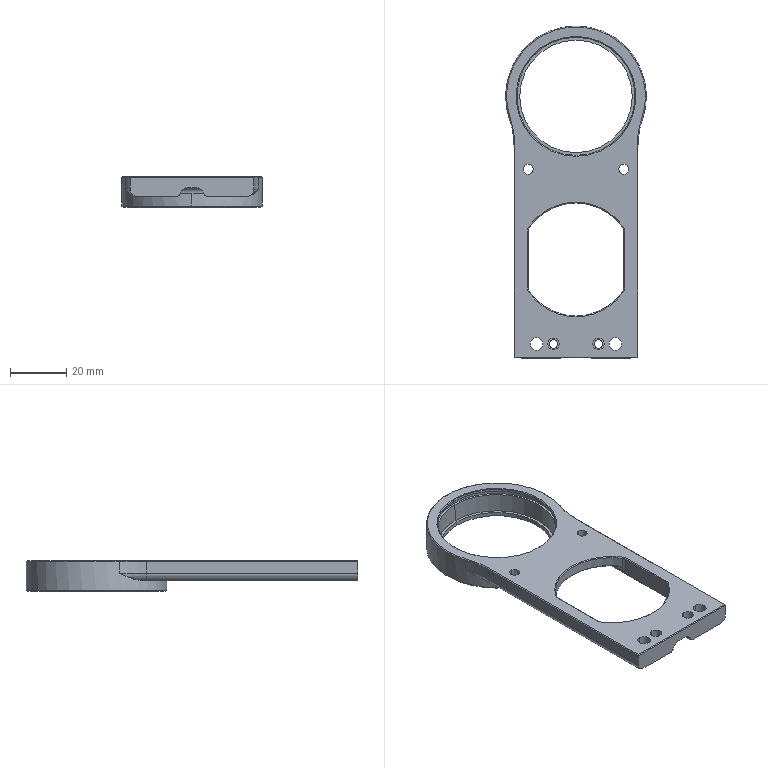NC program | NX | posted with a generic post | part box 50 x 118 x 11 mm
Lines 2350 to 3723 of 3723:
(ZLEVEL_PROFILE_COPY , TOOL : D10JING)
N4680 T14 M6
N4682 G54
N4684 G17 G0 G90 X-64. Y1.257 S9500 M3
N4686 G43 Z30. H14
N4688 Z-9.5
N4690 G94 G1 Y22.549 Z-10.616 F1000.
N4692 X-63.672 Y23.864 Z-10.687
N4694 X-63.004 Y25.045 Z-10.758
N4696 X-62.045 Y26.004 Z-10.829
N4698 X-60.864 Y26.672 Z-10.9
N4700 X-59.549 Y27. Z-10.971
N4702 X-59. Z-11.
N4704 X16.084 F1500.
N4706 G3 X24.227 Y28.364 R25.
N4708 G2 X24.227 Y-28.364 R-30.
N4710 G3 X16.084 Y-27. R25.
N4712 G1 X-59.
N4714 G2 X-64. Y-22. R5.
N4716 G1 Y22.
N4718 G2 X-59. Y27. R5.
N4720 G1 Z-9.5
N4722 G0 Z30.
(ZLEVEL_PROFILE_COPY_1_COPY , TOOL : D10JING)
N4724 X-15.695 Y-12.
N4726 Z-9.
N4728 G1 X-14.834 Z-9.045 F1000.
N4730 X-14.077 Y-11.422 Z-9.095
N4732 X-12.278 Y-9.566 Z-9.231
N4734 X-10.82 Y-7.43 Z-9.366
N4736 X-9.747 Y-5.077 Z-9.502
N4738 X-9.091 Y-2.576 Z-9.637
N4740 X-8.87 Y0. Z-9.773
N4742 X-9.091 Y2.576 Z-9.908
N4744 X-9.747 Y5.077 Z-10.044
N4746 X-10.82 Y7.43 Z-10.179
N4748 X-12.278 Y9.566 Z-10.315
N4750 X-14.077 Y11.422 Z-10.45
N4752 X-14.834 Y12. Z-10.5
N4754 X-33.166 F1500.
N4756 G3 X-33.166 Y-12. R15.1
N4758 G1 X-14.834
N4760 G3 X-14.834 Y12. R15.1
N4762 G1 Z-9.
N4764 G0 Z30.
(HOLE_MILLING_COPY_COPY , TOOL : D10JING)
N4766 X34. Y0.
N4768 Z0.5
N4770 G41 G1 X33.901 Y0.016 F1000. D14
N4772 G3 X34. Y-16.005 R8.011
N4774 X34. Y-16.005 Z-0.5 I0. J16.005 F2000.
N4776 X34. Y-16.005 Z-1.5 I0. J16.005
N4778 X34. Y-16.005 Z-2.5 I0. J16.005
N4780 X34. Y-16.005 Z-3.5 I0. J16.005
N4782 X34. Y-16.005 Z-4.5 I0. J16.005
N4784 X34. Y-16.005 Z-5.5 I0. J16.005
N4786 X34. Y-16.005 Z-6.5 I0. J16.005
N4788 X34. Y-16.005 Z-7.5 I0. J16.005
N4790 X34. Y-16.005 Z-8.5 I0. J16.005
N4792 X34. Y-16.005 Z-9.5 I0. J16.005
N4794 X36.504 Y-15.808 Z-9.525 R16.005
N4796 X49.808 Y2.504 R16.005
N4798 X36.504 Y-15.808 R-16.005
N4800 X34.095 Y0.031 R8.011
N4802 G40
N4804 G1 X34. Y0.
N4806 G0 Z30.
(HOLE_MILLING_COPY_COPY_COPY , TOOL : D10JING)
N4808 Z0.25
N4810 G1 X30.606 Y-11.51 F1000.
N4812 G3 X34. Y-16.05 R3.539
N4814 X34. Y-16.05 Z-0.75 I0. J16.05 F2000.
N4816 X50.05 Y0. Z-1. R16.05
N4818 X34. Y16.05 R16.05
N4820 X50.05 Y0. R-16.05
N4822 X45.51 Y3.394 R3.539
N4824 G1 X34. Y0.
N4826 G0 Z30.
N4828 M5
(SPOT_DRILLING , TOOL : D6A45)
N4830 T01 M6
N4832 G54
N4834 G17 G0 G90 X8.084 Y17. S9500 M3
N4836 G43 Z30. H1
N4838 G94 G82 G98 Z-1. F250. P200 R3.
N4840 X34. Y0.
N4842 X8.084 Y-17.
N4844 X-54. Y-14.
N4846 Y-8.
N4848 Y8.
N4850 Y14.
N4852 G80
N4854 G0 X-54. Y14. Z30.
N4856 M5
(DRILLING , TOOL : 4.5ZT)
N4858 T08 M6
N4860 G54
N4862 G17 G0 G90 X-54. Y14. S2500 M3
N4864 G43 Z30. H8
N4866 G94 G83 G98 Z-6.452 F200. Q2. R3.
N4868 Y-14.
N4870 G80
N4872 G0 X-54. Y-14. Z30.
N4874 M5
(DRILLING_COPY , TOOL : 3.0ZT)
N4876 T16 M6
N4878 G54
N4880 G17 G0 G90 X-54. Y8. S2500 M3
N4882 G43 Z30. H16
N4884 G94 G83 G98 Z-9.401 F200. Q2. R3.
N4886 Y-8.
N4888 G80
N4890 G0 X-54. Y-8. Z30.
N4892 M5
(DRILLING_COPY_COPY , TOOL : 3.5ZT)
N4894 T07 M6
N4896 G54
N4898 G17 G0 G90 X8.084 Y17. S2500 M3
N4900 G43 Z30. H7
N4902 G94 G83 G98 Z-9.521 F200. Q2. R3.
N4904 Y-17.
N4906 G80
N4908 G0 X8.084 Y-17. Z30.
N4910 M5
(ZLEVEL_PROFILE_COPY_1_COPY_1 , TOOL : D4)
N4912 T11 M6
N4914 G54
N4916 G17 G0 G90 X-34.931 Y-13.409 S9500 M3
N4918 G43 Z30. H11
N4920 Z0.808
N4922 G94 G1 Z-0.692 F1000.
N4924 X-35.016 Y-14.113
N4926 G3 X-34.859 Y-14.481 R0.4
N4928 X-34.13 Y-15. R18.1 F2000.
N4930 G1 X-33.269
N4932 G3 X-32.922 Y-14.8 R0.4
N4934 G1 X-32.576 Y-14.2
N4936 Z0.808
N4938 G0 X-34.931 Y-13.409 Z0.415
N4940 G1 Z-1.085 F1000.
N4942 X-35.016 Y-14.113
N4944 G3 X-34.859 Y-14.481 R0.4
N4946 X-34.13 Y-15. R18.1 F2000.
N4948 G1 X-33.269
N4950 G3 X-32.922 Y-14.8 R0.4
N4952 G1 X-32.576 Y-14.2
N4954 Z0.415
N4956 G0 X-34.931 Y-13.409 Z0.023
N4958 G1 Z-1.477 F1000.
N4960 X-35.016 Y-14.113
N4962 G3 X-34.859 Y-14.481 R0.4
N4964 X-34.13 Y-15. R18.1 F2000.
N4966 G1 X-33.269
N4968 G3 X-32.922 Y-14.8 R0.4
N4970 G1 X-32.576 Y-14.2
N4972 Z0.023
N4974 G0 X-34.931 Y-13.409 Z-0.369
N4976 G1 Z-1.869 F1000.
N4978 X-35.016 Y-14.113
N4980 G3 X-34.859 Y-14.481 R0.4
N4982 X-34.13 Y-15. R18.1 F2000.
N4984 G1 X-33.269
N4986 G3 X-32.922 Y-14.8 R0.4
N4988 G1 X-32.576 Y-14.2
N4990 Z-0.369
N4992 G0 X-34.931 Y-13.409 Z-0.762
N4994 G1 Z-2.262 F1000.
N4996 X-35.016 Y-14.113
N4998 G3 X-34.859 Y-14.481 R0.4
N5000 X-34.13 Y-15. R18.1 F2000.
N5002 G1 X-33.269
N5004 G3 X-32.922 Y-14.8 R0.4
N5006 G1 X-32.576 Y-14.2
N5008 Z-0.762
N5010 G0 X-34.931 Y-13.409 Z-1.154
N5012 G1 Z-2.654 F1000.
N5014 X-35.016 Y-14.113
N5016 G3 X-34.859 Y-14.481 R0.4
N5018 X-34.13 Y-15. R18.1 F2000.
N5020 G1 X-33.269
N5022 G3 X-32.922 Y-14.8 R0.4
N5024 G1 X-32.576 Y-14.2
N5026 Z-1.154
N5028 G0 X-34.931 Y-13.409 Z-1.546
N5030 G1 Z-3.046 F1000.
N5032 X-35.016 Y-14.113
N5034 G3 X-34.859 Y-14.481 R0.4
N5036 X-34.13 Y-15. R18.1 F2000.
N5038 G1 X-33.269
N5040 G3 X-32.922 Y-14.8 R0.4
N5042 G1 X-32.576 Y-14.2
N5044 Z-1.546
N5046 G0 X-34.931 Y-13.409 Z-1.938
N5048 G1 Z-3.438 F1000.
N5050 X-35.016 Y-14.113
N5052 G3 X-34.859 Y-14.481 R0.4
N5054 X-34.13 Y-15. R18.1 F2000.
N5056 G1 X-33.269
N5058 G3 X-32.922 Y-14.8 R0.4
N5060 G1 X-32.576 Y-14.2
N5062 Z-1.938
N5064 G0 X-34.931 Y-13.409 Z-2.331
N5066 G1 Z-3.831 F1000.
N5068 X-35.016 Y-14.113
N5070 G3 X-34.859 Y-14.481 R0.4
N5072 X-34.13 Y-15. R18.1 F2000.
N5074 G1 X-33.269
N5076 G3 X-32.922 Y-14.8 R0.4
N5078 G1 X-32.576 Y-14.2
N5080 Z-2.331
N5082 G0 X-34.931 Y-13.409 Z-2.723
N5084 G1 Z-4.223 F1000.
N5086 X-35.016 Y-14.113
N5088 G3 X-34.859 Y-14.481 R0.4
N5090 X-34.13 Y-15. R18.1 F2000.
N5092 G1 X-33.269
N5094 G3 X-32.922 Y-14.8 R0.4
N5096 G1 X-32.576 Y-14.2
N5098 Z-2.723
N5100 G0 X-34.931 Y-13.409 Z-3.115
N5102 G1 Z-4.615 F1000.
N5104 X-35.016 Y-14.113
N5106 G3 X-34.859 Y-14.481 R0.4
N5108 X-34.13 Y-15. R18.1 F2000.
N5110 G1 X-33.269
N5112 G3 X-32.922 Y-14.8 R0.4
N5114 G1 X-32.576 Y-14.2
N5116 Z-3.115
N5118 G0 X-34.931 Y-13.409 Z-3.508
N5120 G1 Z-5.008 F1000.
N5122 X-35.016 Y-14.113
N5124 G3 X-34.859 Y-14.481 R0.4
N5126 X-34.13 Y-15. R18.1 F2000.
N5128 G1 X-33.269
N5130 G3 X-32.922 Y-14.8 R0.4
N5132 G1 X-32.576 Y-14.2
N5134 Z-3.508
N5136 G0 X-34.931 Y-13.409 Z-3.9
N5138 G1 Z-5.4 F1000.
N5140 X-35.016 Y-14.113
N5142 G3 X-34.859 Y-14.481 R0.4
N5144 X-34.13 Y-15. R18.1 F2000.
N5146 G1 X-33.269
N5148 G3 X-32.922 Y-14.8 R0.4
N5150 G1 X-32.576 Y-14.2
N5152 Z-3.9
N5154 G0 X-34.931 Y-13.409 Z-4.292
N5156 G1 Z-5.792 F1000.
N5158 X-35.016 Y-14.113
N5160 G3 X-34.859 Y-14.481 R0.4
N5162 X-34.13 Y-15. R18.1 F2000.
N5164 G1 X-33.269
N5166 G3 X-32.922 Y-14.8 R0.4
N5168 G1 X-32.576 Y-14.2
N5170 Z-4.292
N5172 G0 X-34.931 Y-13.409 Z-4.685
N5174 G1 Z-6.185 F1000.
N5176 X-35.016 Y-14.113
N5178 G3 X-34.859 Y-14.481 R0.4
N5180 X-34.13 Y-15. R18.1 F2000.
N5182 G1 X-33.269
N5184 G3 X-32.922 Y-14.8 R0.4
N5186 G1 X-32.576 Y-14.2
N5188 Z-4.685
N5190 G0 X-34.931 Y-13.409 Z-5.077
N5192 G1 Z-6.577 F1000.
N5194 X-35.016 Y-14.113
N5196 G3 X-34.859 Y-14.481 R0.4
N5198 X-34.13 Y-15. R18.1 F2000.
N5200 G1 X-33.269
N5202 G3 X-32.922 Y-14.8 R0.4
N5204 G1 X-32.576 Y-14.2
N5206 Z-5.077
N5208 G0 X-34.939 Y-13.403 Z-5.469
N5210 G1 Z-6.969 F1000.
N5212 X-35.024 Y-14.107
N5214 G3 X-34.867 Y-14.475 R0.4
N5216 X-34.135 Y-14.997 R18.1 F2000.
N5218 G1 X-34.089 Y-15.
N5220 X-33.265
N5222 G3 X-32.918 Y-14.8 R0.4
N5224 G1 X-32.572 Y-14.2
N5226 Z-5.469
N5228 G0 X-34.939 Y-13.403 Z-5.862
N5230 G1 Z-7.362 F1000.
N5232 X-35.024 Y-14.107
N5234 G3 X-34.867 Y-14.475 R0.4
N5236 X-34.135 Y-14.997 R18.1 F2000.
N5238 G1 X-34.089 Y-15.
N5240 X-33.265
N5242 G3 X-32.918 Y-14.8 R0.4
N5244 G1 X-32.572 Y-14.2
N5246 Z-5.862
N5248 G0 X-34.939 Y-13.403 Z-6.254
N5250 G1 Z-7.754 F1000.
N5252 X-35.024 Y-14.107
N5254 G3 X-34.867 Y-14.475 R0.4
N5256 X-34.135 Y-14.997 R18.1 F2000.
N5258 G1 X-34.089 Y-15.
N5260 X-33.265
N5262 G3 X-32.918 Y-14.8 R0.4
N5264 G1 X-32.572 Y-14.2
N5266 Z-6.254
N5268 G0 X-34.939 Y-13.403 Z-6.646
N5270 G1 Z-8.146 F1000.
N5272 X-35.024 Y-14.107
N5274 G3 X-34.867 Y-14.475 R0.4
N5276 X-34.135 Y-14.997 R18.1 F2000.
N5278 G1 X-34.089 Y-15.
N5280 X-33.265
N5282 G3 X-32.918 Y-14.8 R0.4
N5284 G1 X-32.572 Y-14.2
N5286 Z-6.646
N5288 G0 X-34.939 Y-13.403 Z-7.038
N5290 G1 Z-8.538 F1000.
N5292 X-35.024 Y-14.107
N5294 G3 X-34.867 Y-14.475 R0.4
N5296 X-34.135 Y-14.997 R18.1 F2000.
N5298 G1 X-34.089 Y-15.
N5300 X-33.265
N5302 G3 X-32.918 Y-14.8 R0.4
N5304 G1 X-32.572 Y-14.2
N5306 Z-7.038
N5308 G0 X-34.939 Y-13.403 Z-7.431
N5310 G1 Z-8.931 F1000.
N5312 X-35.024 Y-14.107
N5314 G3 X-34.867 Y-14.475 R0.4
N5316 X-34.135 Y-14.997 R18.1 F2000.
N5318 G1 X-34.089 Y-15.
N5320 X-33.265
N5322 G3 X-32.918 Y-14.8 R0.4
N5324 G1 X-32.572 Y-14.2
N5326 Z-7.431
N5328 G0 X-34.939 Y-13.403 Z-7.823
N5330 G1 Z-9.323 F1000.
N5332 X-35.024 Y-14.107
N5334 G3 X-34.867 Y-14.475 R0.4
N5336 X-34.135 Y-14.997 R18.1 F2000.
N5338 G1 X-34.089 Y-15.
N5340 X-33.265
N5342 G3 X-32.918 Y-14.8 R0.4
N5344 G1 X-32.572 Y-14.2
N5346 Z-7.823
N5348 G0 X-34.939 Y-13.403 Z-8.215
N5350 G1 Z-9.715 F1000.
N5352 X-35.024 Y-14.107
N5354 G3 X-34.867 Y-14.475 R0.4
N5356 X-34.135 Y-14.997 R18.1 F2000.
N5358 G1 X-34.089 Y-15.
N5360 X-33.265
N5362 G3 X-32.918 Y-14.8 R0.4
N5364 G1 X-32.572 Y-14.2
N5366 Z-8.215
N5368 G0 X-34.939 Y-13.403 Z-8.608
N5370 G1 Z-10.108 F1000.
N5372 X-35.024 Y-14.107
N5374 G3 X-34.867 Y-14.475 R0.4
N5376 X-34.135 Y-14.997 R18.1 F2000.
N5378 G1 X-34.089 Y-15.
N5380 X-33.265
N5382 G3 X-32.918 Y-14.8 R0.4
N5384 G1 X-32.572 Y-14.2
N5386 Z-8.608
N5388 G0 X-34.939 Y-13.403 Z-9.
N5390 G1 Z-10.5 F1000.
N5392 X-35.024 Y-14.107
N5394 G3 X-34.867 Y-14.475 R0.4
N5396 X-34.135 Y-14.997 R18.1 F2000.
N5398 G1 X-34.089 Y-15.
N5400 X-33.265
N5402 G3 X-32.918 Y-14.8 R0.4
N5404 G1 X-32.572 Y-14.2
N5406 Z-9.
N5408 G0 Z30.
N5410 X-15.424
N5412 Z0.808
N5414 G1 Z-0.692 F1000.
N5416 X-15.078 Y-14.8
N5418 G3 X-14.731 Y-15. R0.4
N5420 G1 X-13.87 F2000.
N5422 G3 X-13.141 Y-14.481 R18.1
N5424 X-12.984 Y-14.113 R0.4
N5426 G1 X-13.069 Y-13.409
N5428 Z0.808
N5430 G0 X-15.424 Y-14.2 Z0.415
N5432 G1 Z-1.085 F1000.
N5434 X-15.078 Y-14.8
N5436 G3 X-14.731 Y-15. R0.4
N5438 G1 X-13.87 F2000.
N5440 G3 X-13.141 Y-14.481 R18.1
N5442 X-12.984 Y-14.113 R0.4
N5444 G1 X-13.069 Y-13.409
N5446 Z0.415
N5448 G0 X-15.424 Y-14.2 Z0.023
N5450 G1 Z-1.477 F1000.
N5452 X-15.078 Y-14.8
N5454 G3 X-14.731 Y-15. R0.4
N5456 G1 X-13.87 F2000.
N5458 G3 X-13.141 Y-14.481 R18.1
N5460 X-12.984 Y-14.113 R0.4
N5462 G1 X-13.069 Y-13.409
N5464 Z0.023
N5466 G0 X-15.424 Y-14.2 Z-0.369
N5468 G1 Z-1.869 F1000.
N5470 X-15.078 Y-14.8
N5472 G3 X-14.731 Y-15. R0.4
N5474 G1 X-13.87 F2000.
N5476 G3 X-13.141 Y-14.481 R18.1
N5478 X-12.984 Y-14.113 R0.4
N5480 G1 X-13.069 Y-13.409
N5482 Z-0.369
N5484 G0 X-15.424 Y-14.2 Z-0.762
N5486 G1 Z-2.262 F1000.
N5488 X-15.078 Y-14.8
N5490 G3 X-14.731 Y-15. R0.4
N5492 G1 X-13.87 F2000.
N5494 G3 X-13.141 Y-14.481 R18.1
N5496 X-12.984 Y-14.113 R0.4
N5498 G1 X-13.069 Y-13.409
N5500 Z-0.762
N5502 G0 X-15.424 Y-14.2 Z-1.154
N5504 G1 Z-2.654 F1000.
N5506 X-15.078 Y-14.8
N5508 G3 X-14.731 Y-15. R0.4
N5510 G1 X-13.87 F2000.
N5512 G3 X-13.141 Y-14.481 R18.1
N5514 X-12.984 Y-14.113 R0.4
N5516 G1 X-13.069 Y-13.409
N5518 Z-1.154
N5520 G0 X-15.424 Y-14.2 Z-1.546
N5522 G1 Z-3.046 F1000.
N5524 X-15.078 Y-14.8
N5526 G3 X-14.731 Y-15. R0.4
N5528 G1 X-13.87 F2000.
N5530 G3 X-13.141 Y-14.481 R18.1
N5532 X-12.984 Y-14.113 R0.4
N5534 G1 X-13.069 Y-13.409
N5536 Z-1.546
N5538 G0 X-15.424 Y-14.2 Z-1.938
N5540 G1 Z-3.438 F1000.
N5542 X-15.078 Y-14.8
N5544 G3 X-14.731 Y-15. R0.4
N5546 G1 X-13.87 F2000.
N5548 G3 X-13.141 Y-14.481 R18.1
N5550 X-12.984 Y-14.113 R0.4
N5552 G1 X-13.069 Y-13.409
N5554 Z-1.938
N5556 G0 X-15.424 Y-14.2 Z-2.331
N5558 G1 Z-3.831 F1000.
N5560 X-15.078 Y-14.8
N5562 G3 X-14.731 Y-15. R0.4
N5564 G1 X-13.87 F2000.
N5566 G3 X-13.141 Y-14.481 R18.1
N5568 X-12.984 Y-14.113 R0.4
N5570 G1 X-13.069 Y-13.409
N5572 Z-2.331
N5574 G0 X-15.424 Y-14.2 Z-2.723
N5576 G1 Z-4.223 F1000.
N5578 X-15.078 Y-14.8
N5580 G3 X-14.731 Y-15. R0.4
N5582 G1 X-13.87 F2000.
N5584 G3 X-13.141 Y-14.481 R18.1
N5586 X-12.984 Y-14.113 R0.4
N5588 G1 X-13.069 Y-13.409
N5590 Z-2.723
N5592 G0 X-15.424 Y-14.2 Z-3.115
N5594 G1 Z-4.615 F1000.
N5596 X-15.078 Y-14.8
N5598 G3 X-14.731 Y-15. R0.4
N5600 G1 X-13.87 F2000.
N5602 G3 X-13.141 Y-14.481 R18.1
N5604 X-12.984 Y-14.113 R0.4
N5606 G1 X-13.069 Y-13.409
N5608 Z-3.115
N5610 G0 X-15.424 Y-14.2 Z-3.508
N5612 G1 Z-5.008 F1000.
N5614 X-15.078 Y-14.8
N5616 G3 X-14.731 Y-15. R0.4
N5618 G1 X-13.87 F2000.
N5620 X-13.863 Y-14.995
N5622 G3 X-13.141 Y-14.481 R18.1
N5624 X-12.984 Y-14.113 R0.4
N5626 G1 X-13.069 Y-13.409
N5628 Z-3.508
N5630 G0 X-15.424 Y-14.2 Z-3.9
N5632 G1 Z-5.4 F1000.
N5634 X-15.078 Y-14.8
N5636 G3 X-14.731 Y-15. R0.4
N5638 G1 X-13.871 F2000.
N5640 X-13.867 Y-14.998
N5642 G3 X-13.141 Y-14.481 R18.1
N5644 X-12.984 Y-14.113 R0.4
N5646 G1 X-13.069 Y-13.409
N5648 Z-3.9
N5650 G0 X-15.424 Y-14.2 Z-4.292
N5652 G1 Z-5.792 F1000.
N5654 X-15.078 Y-14.8
N5656 G3 X-14.731 Y-15. R0.4
N5658 G1 X-13.868 Y-14.998 F2000.
N5660 G3 X-13.141 Y-14.481 R18.1
N5662 X-12.984 Y-14.113 R0.4
N5664 G1 X-13.069 Y-13.409
N5666 Z-4.292
N5668 G0 X-15.424 Y-14.2 Z-4.685
N5670 G1 Z-6.185 F1000.
N5672 X-15.078 Y-14.8
N5674 G3 X-14.731 Y-15. R0.4
N5676 G1 X-13.871 F2000.
N5678 X-13.868 Y-14.998
N5680 G3 X-13.141 Y-14.481 R18.1
N5682 X-12.984 Y-14.113 R0.4
N5684 G1 X-13.069 Y-13.409
N5686 Z-4.685
N5688 G0 X-15.424 Y-14.2 Z-5.077
N5690 G1 Z-6.577 F1000.
N5692 X-15.078 Y-14.8
N5694 G3 X-14.731 Y-15. R0.4
N5696 G1 X-13.906 F2000.
N5698 X-13.868 Y-14.999
N5700 G3 X-13.141 Y-14.481 R18.1
N5702 X-12.984 Y-14.113 R0.4
N5704 G1 X-13.069 Y-13.409
N5706 Z-5.077
N5708 G0 X-15.421 Y-14.2 Z-5.469
N5710 G1 Z-6.969 F1000.
N5712 X-15.075 Y-14.8
N5714 G3 X-14.728 Y-15. R0.4
N5716 G1 X-13.868 Y-14.999 F2000.
N5718 G3 X-13.146 Y-14.485 R18.1
N5720 X-12.989 Y-14.117 R0.4
N5722 G1 X-13.074 Y-13.413
N5724 Z-5.469
N5726 G0 X-15.421 Y-14.2 Z-5.862
N5728 G1 Z-7.362 F1000.
N5730 X-15.075 Y-14.8
N5732 G3 X-14.728 Y-15. R0.4
N5734 G1 X-13.868 Y-14.999 F2000.
N5736 G3 X-13.146 Y-14.485 R18.1
N5738 X-12.989 Y-14.117 R0.4
N5740 G1 X-13.074 Y-13.413
N5742 Z-5.862
N5744 G0 X-15.421 Y-14.2 Z-6.254
N5746 G1 Z-7.754 F1000.
N5748 X-15.075 Y-14.8
N5750 G3 X-14.728 Y-15. R0.4
N5752 G1 X-13.868 Y-14.999 F2000.
N5754 G3 X-13.146 Y-14.485 R18.1
N5756 X-12.989 Y-14.117 R0.4
N5758 G1 X-13.074 Y-13.413
N5760 Z-6.254
N5762 G0 X-15.421 Y-14.2 Z-6.646
N5764 G1 Z-8.146 F1000.
N5766 X-15.075 Y-14.8
N5768 G3 X-14.728 Y-15. R0.4
N5770 G1 X-13.868 Y-14.999 F2000.
N5772 G3 X-13.146 Y-14.485 R18.1
N5774 X-12.989 Y-14.117 R0.4
N5776 G1 X-13.074 Y-13.413
N5778 Z-6.646
N5780 G0 X-15.421 Y-14.2 Z-7.038
N5782 G1 Z-8.538 F1000.
N5784 X-15.075 Y-14.8
N5786 G3 X-14.728 Y-15. R0.4
N5788 G1 X-13.868 Y-14.999 F2000.
N5790 G3 X-13.146 Y-14.485 R18.1
N5792 X-12.989 Y-14.117 R0.4
N5794 G1 X-13.074 Y-13.413
N5796 Z-7.038
N5798 G0 X-15.421 Y-14.2 Z-7.431
N5800 G1 Z-8.931 F1000.
N5802 X-15.075 Y-14.8
N5804 G3 X-14.728 Y-15. R0.4
N5806 G1 X-13.868 Y-14.999 F2000.
N5808 G3 X-13.146 Y-14.485 R18.1
N5810 X-12.989 Y-14.117 R0.4
N5812 G1 X-13.074 Y-13.413
N5814 Z-7.431
N5816 G0 X-15.421 Y-14.2 Z-7.823
N5818 G1 Z-9.323 F1000.
N5820 X-15.075 Y-14.8
N5822 G3 X-14.728 Y-15. R0.4
N5824 G1 X-13.868 Y-14.999 F2000.
N5826 G3 X-13.146 Y-14.485 R18.1
N5828 X-12.989 Y-14.117 R0.4
N5830 G1 X-13.074 Y-13.413
N5832 Z-7.823
N5834 G0 X-15.421 Y-14.2 Z-8.215
N5836 G1 Z-9.715 F1000.
N5838 X-15.075 Y-14.8
N5840 G3 X-14.728 Y-15. R0.4
N5842 G1 X-13.868 Y-14.999 F2000.
N5844 G3 X-13.146 Y-14.485 R18.1
N5846 X-12.989 Y-14.117 R0.4
N5848 G1 X-13.074 Y-13.413
N5850 Z-8.215
N5852 G0 X-15.421 Y-14.2 Z-8.608
N5854 G1 Z-10.108 F1000.
N5856 X-15.075 Y-14.8
N5858 G3 X-14.728 Y-15. R0.4
N5860 G1 X-13.868 Y-14.999 F2000.
N5862 G3 X-13.146 Y-14.485 R18.1
N5864 X-12.989 Y-14.117 R0.4
N5866 G1 X-13.074 Y-13.413
N5868 Z-8.608
N5870 G0 X-15.421 Y-14.2 Z-9.
N5872 G1 Z-10.5 F1000.
N5874 X-15.075 Y-14.8
N5876 G3 X-14.728 Y-15. R0.4
N5878 G1 X-13.868 Y-14.999 F2000.
N5880 G3 X-13.146 Y-14.485 R18.1
N5882 X-12.989 Y-14.117 R0.4
N5884 G1 X-13.074 Y-13.413
N5886 Z-9.
N5888 G0 Z30.
N5890 X-13.069 Y13.409
N5892 Z0.808
N5894 G1 Z-0.692 F1000.
N5896 X-12.984 Y14.113
N5898 G3 X-13.141 Y14.481 R0.4
N5900 X-13.87 Y15. R18.1 F2000.
N5902 G1 X-14.731
N5904 G3 X-15.078 Y14.8 R0.4
N5906 G1 X-15.424 Y14.2
N5908 Z0.808
N5910 G0 X-13.069 Y13.409 Z0.415
N5912 G1 Z-1.085 F1000.
N5914 X-12.984 Y14.113
N5916 G3 X-13.141 Y14.481 R0.4
N5918 X-13.87 Y15. R18.1 F2000.
N5920 G1 X-14.731
N5922 G3 X-15.078 Y14.8 R0.4
N5924 G1 X-15.424 Y14.2
N5926 Z0.415
N5928 G0 X-13.069 Y13.409 Z0.023
N5930 G1 Z-1.477 F1000.
N5932 X-12.984 Y14.113
N5934 G3 X-13.141 Y14.481 R0.4
N5936 X-13.87 Y15. R18.1 F2000.
N5938 G1 X-14.731
N5940 G3 X-15.078 Y14.8 R0.4
N5942 G1 X-15.424 Y14.2
N5944 Z0.023
N5946 G0 X-13.069 Y13.409 Z-0.369
N5948 G1 Z-1.869 F1000.
N5950 X-12.984 Y14.113
N5952 G3 X-13.141 Y14.481 R0.4
N5954 X-13.87 Y15. R18.1 F2000.
N5956 G1 X-14.731
N5958 G3 X-15.078 Y14.8 R0.4
N5960 G1 X-15.424 Y14.2
N5962 Z-0.369
N5964 G0 X-13.069 Y13.409 Z-0.762
N5966 G1 Z-2.262 F1000.
N5968 X-12.984 Y14.113
N5970 G3 X-13.141 Y14.481 R0.4
N5972 X-13.87 Y15. R18.1 F2000.
N5974 G1 X-14.731
N5976 G3 X-15.078 Y14.8 R0.4
N5978 G1 X-15.424 Y14.2
N5980 Z-0.762
N5982 G0 X-13.069 Y13.409 Z-1.154
N5984 G1 Z-2.654 F1000.
N5986 X-12.984 Y14.113
N5988 G3 X-13.141 Y14.481 R0.4
N5990 X-13.87 Y15. R18.1 F2000.
N5992 G1 X-14.731
N5994 G3 X-15.078 Y14.8 R0.4
N5996 G1 X-15.424 Y14.2
N5998 Z-1.154
N6000 G0 X-13.069 Y13.409 Z-1.546
N6002 G1 Z-3.046 F1000.
N6004 X-12.984 Y14.113
N6006 G3 X-13.141 Y14.481 R0.4
N6008 X-13.87 Y15. R18.1 F2000.
N6010 G1 X-14.731
N6012 G3 X-15.078 Y14.8 R0.4
N6014 G1 X-15.424 Y14.2
N6016 Z-1.546
N6018 G0 X-13.069 Y13.409 Z-1.938
N6020 G1 Z-3.438 F1000.
N6022 X-12.984 Y14.113
N6024 G3 X-13.141 Y14.481 R0.4
N6026 X-13.87 Y15. R18.1 F2000.
N6028 G1 X-14.731
N6030 G3 X-15.078 Y14.8 R0.4
N6032 G1 X-15.424 Y14.2
N6034 Z-1.938
N6036 G0 X-13.069 Y13.409 Z-2.331
N6038 G1 Z-3.831 F1000.
N6040 X-12.984 Y14.113
N6042 G3 X-13.141 Y14.481 R0.4
N6044 X-13.87 Y15. R18.1 F2000.
N6046 G1 X-14.731
N6048 G3 X-15.078 Y14.8 R0.4
N6050 G1 X-15.424 Y14.2
N6052 Z-2.331
N6054 G0 X-13.069 Y13.409 Z-2.723
N6056 G1 Z-4.223 F1000.
N6058 X-12.984 Y14.113
N6060 G3 X-13.141 Y14.481 R0.4
N6062 X-13.87 Y15. R18.1 F2000.
N6064 G1 X-14.731
N6066 G3 X-15.078 Y14.8 R0.4
N6068 G1 X-15.424 Y14.2
N6070 Z-2.723
N6072 G0 X-13.069 Y13.409 Z-3.115
N6074 G1 Z-4.615 F1000.
N6076 X-12.984 Y14.113
N6078 G3 X-13.141 Y14.481 R0.4
N6080 X-13.87 Y15. R18.1 F2000.
N6082 G1 X-14.731
N6084 G3 X-15.078 Y14.8 R0.4
N6086 G1 X-15.424 Y14.2
N6088 Z-3.115
N6090 G0 X-13.069 Y13.409 Z-3.508
N6092 G1 Z-5.008 F1000.
N6094 X-12.984 Y14.113
N6096 G3 X-13.141 Y14.481 R0.4
N6098 X-13.871 Y15. R18.1 F2000.
N6100 G1 X-14.731
N6102 G3 X-15.078 Y14.8 R0.4
N6104 G1 X-15.424 Y14.2
N6106 Z-3.508
N6108 G0 X-13.069 Y13.409 Z-3.9
N6110 G1 Z-5.4 F1000.
N6112 X-12.984 Y14.113
N6114 G3 X-13.141 Y14.481 R0.4
N6116 X-13.871 Y15. R18.1 F2000.
N6118 G1 X-14.731
N6120 G3 X-15.078 Y14.8 R0.4
N6122 G1 X-15.424 Y14.2
N6124 Z-3.9
N6126 G0 X-13.069 Y13.409 Z-4.292
N6128 G1 Z-5.792 F1000.
N6130 X-12.984 Y14.113
N6132 G3 X-13.141 Y14.481 R0.4
N6134 X-13.871 Y15. R18.1 F2000.
N6136 G1 X-14.731
N6138 G3 X-15.078 Y14.8 R0.4
N6140 G1 X-15.424 Y14.2
N6142 Z-4.292
N6144 G0 X-13.069 Y13.409 Z-4.685
N6146 G1 Z-6.185 F1000.
N6148 X-12.984 Y14.113
N6150 G3 X-13.141 Y14.481 R0.4
N6152 X-13.868 Y14.998 R18.1 F2000.
N6154 G1 X-13.871 Y15.
N6156 X-14.731
N6158 G3 X-15.078 Y14.8 R0.4
N6160 G1 X-15.424 Y14.2
N6162 Z-4.685
N6164 G0 X-13.069 Y13.409 Z-5.077
N6166 G1 Z-6.577 F1000.
N6168 X-12.984 Y14.113
N6170 G3 X-13.141 Y14.481 R0.4
N6172 X-13.868 Y14.998 R18.1 F2000.
N6174 G1 X-13.909 Y15.
N6176 X-14.731
N6178 G3 X-15.078 Y14.8 R0.4
N6180 G1 X-15.424 Y14.2
N6182 Z-5.077
N6184 G0 X-13.074 Y13.413 Z-5.469
N6186 G1 Z-6.969 F1000.
N6188 X-12.989 Y14.117
N6190 G3 X-13.146 Y14.485 R0.4
N6192 X-13.868 Y14.999 R18.1 F2000.
N6194 G1 X-14.728 Y15.
N6196 G3 X-15.075 Y14.8 R0.4
N6198 G1 X-15.421 Y14.2
N6200 Z-5.469
N6202 G0 X-13.074 Y13.413 Z-5.862
N6204 G1 Z-7.362 F1000.
N6206 X-12.989 Y14.117
N6208 G3 X-13.146 Y14.485 R0.4
N6210 X-13.868 Y14.999 R18.1 F2000.
N6212 G1 X-14.728 Y15.
N6214 G3 X-15.075 Y14.8 R0.4
N6216 G1 X-15.421 Y14.2
N6218 Z-5.862
N6220 G0 X-13.074 Y13.413 Z-6.254
N6222 G1 Z-7.754 F1000.
N6224 X-12.989 Y14.117
N6226 G3 X-13.146 Y14.485 R0.4
N6228 X-13.868 Y14.999 R18.1 F2000.
N6230 G1 X-14.728 Y15.
N6232 G3 X-15.075 Y14.8 R0.4
N6234 G1 X-15.421 Y14.2
N6236 Z-6.254
N6238 G0 X-13.074 Y13.413 Z-6.646
N6240 G1 Z-8.146 F1000.
N6242 X-12.989 Y14.117
N6244 G3 X-13.146 Y14.485 R0.4
N6246 X-13.868 Y14.999 R18.1 F2000.
N6248 G1 X-14.728 Y15.
N6250 G3 X-15.075 Y14.8 R0.4
N6252 G1 X-15.421 Y14.2
N6254 Z-6.646
N6256 G0 X-13.074 Y13.413 Z-7.038
N6258 G1 Z-8.538 F1000.
N6260 X-12.989 Y14.117
N6262 G3 X-13.146 Y14.485 R0.4
N6264 X-13.868 Y14.999 R18.1 F2000.
N6266 G1 X-14.728 Y15.
N6268 G3 X-15.075 Y14.8 R0.4
N6270 G1 X-15.421 Y14.2
N6272 Z-7.038
N6274 G0 X-13.074 Y13.413 Z-7.431
N6276 G1 Z-8.931 F1000.
N6278 X-12.989 Y14.117
N6280 G3 X-13.146 Y14.485 R0.4
N6282 X-13.868 Y14.999 R18.1 F2000.
N6284 G1 X-14.728 Y15.
N6286 G3 X-15.075 Y14.8 R0.4
N6288 G1 X-15.421 Y14.2
N6290 Z-7.431
N6292 G0 X-13.074 Y13.413 Z-7.823
N6294 G1 Z-9.323 F1000.
N6296 X-12.989 Y14.117
N6298 G3 X-13.146 Y14.485 R0.4
N6300 X-13.868 Y14.999 R18.1 F2000.
N6302 G1 X-14.728 Y15.
N6304 G3 X-15.075 Y14.8 R0.4
N6306 G1 X-15.421 Y14.2
N6308 Z-7.823
N6310 G0 X-13.074 Y13.413 Z-8.215
N6312 G1 Z-9.715 F1000.
N6314 X-12.989 Y14.117
N6316 G3 X-13.146 Y14.485 R0.4
N6318 X-13.868 Y14.999 R18.1 F2000.
N6320 G1 X-14.728 Y15.
N6322 G3 X-15.075 Y14.8 R0.4
N6324 G1 X-15.421 Y14.2
N6326 Z-8.215
N6328 G0 X-13.074 Y13.413 Z-8.608
N6330 G1 Z-10.108 F1000.
N6332 X-12.989 Y14.117
N6334 G3 X-13.146 Y14.485 R0.4
N6336 X-13.868 Y14.999 R18.1 F2000.
N6338 G1 X-14.728 Y15.
N6340 G3 X-15.075 Y14.8 R0.4
N6342 G1 X-15.421 Y14.2
N6344 Z-8.608
N6346 G0 X-13.074 Y13.413 Z-9.
N6348 G1 Z-10.5 F1000.
N6350 X-12.989 Y14.117
N6352 G3 X-13.146 Y14.485 R0.4
N6354 X-13.868 Y14.999 R18.1 F2000.
N6356 G1 X-14.728 Y15.
N6358 G3 X-15.075 Y14.8 R0.4
N6360 G1 X-15.421 Y14.2
N6362 Z-9.
N6364 G0 Z30.
N6366 X-32.576
N6368 Z0.808
N6370 G1 Z-0.692 F1000.
N6372 X-32.922 Y14.8
N6374 G3 X-33.269 Y15. R0.4
N6376 G1 X-34.13 F2000.
N6378 G3 X-34.859 Y14.481 R18.1
N6380 X-35.016 Y14.113 R0.4
N6382 G1 X-34.931 Y13.409
N6384 Z0.808
N6386 G0 X-32.576 Y14.2 Z0.415
N6388 G1 Z-1.085 F1000.
N6390 X-32.922 Y14.8
N6392 G3 X-33.269 Y15. R0.4
N6394 G1 X-34.13 F2000.
N6396 G3 X-34.859 Y14.481 R18.1
N6398 X-35.016 Y14.113 R0.4
N6400 G1 X-34.931 Y13.409
N6402 Z0.415
N6404 G0 X-32.576 Y14.2 Z0.023
N6406 G1 Z-1.477 F1000.
N6408 X-32.922 Y14.8
N6410 G3 X-33.269 Y15. R0.4
N6412 G1 X-34.13 F2000.
N6414 G3 X-34.859 Y14.481 R18.1
N6416 X-35.016 Y14.113 R0.4
N6418 G1 X-34.931 Y13.409
N6420 Z0.023
N6422 G0 X-32.576 Y14.2 Z-0.369
N6424 G1 Z-1.869 F1000.
N6426 X-32.922 Y14.8
N6428 G3 X-33.269 Y15. R0.4
N6430 G1 X-34.13 F2000.
N6432 G3 X-34.859 Y14.481 R18.1
N6434 X-35.016 Y14.113 R0.4
N6436 G1 X-34.931 Y13.409
N6438 Z-0.369
N6440 G0 X-32.576 Y14.2 Z-0.762
N6442 G1 Z-2.262 F1000.
N6444 X-32.922 Y14.8
N6446 G3 X-33.269 Y15. R0.4
N6448 G1 X-34.13 F2000.
N6450 G3 X-34.859 Y14.481 R18.1
N6452 X-35.016 Y14.113 R0.4
N6454 G1 X-34.931 Y13.409
N6456 Z-0.762
N6458 G0 X-32.576 Y14.2 Z-1.154
N6460 G1 Z-2.654 F1000.
N6462 X-32.922 Y14.8
N6464 G3 X-33.269 Y15. R0.4
N6466 G1 X-34.13 F2000.
N6468 G3 X-34.859 Y14.481 R18.1
N6470 X-35.016 Y14.113 R0.4
N6472 G1 X-34.931 Y13.409
N6474 Z-1.154
N6476 G0 X-32.576 Y14.2 Z-1.546
N6478 G1 Z-3.046 F1000.
N6480 X-32.922 Y14.8
N6482 G3 X-33.269 Y15. R0.4
N6484 G1 X-34.13 F2000.
N6486 G3 X-34.859 Y14.481 R18.1
N6488 X-35.016 Y14.113 R0.4
N6490 G1 X-34.931 Y13.409
N6492 Z-1.546
N6494 G0 X-32.576 Y14.2 Z-1.938
N6496 G1 Z-3.438 F1000.
N6498 X-32.922 Y14.8
N6500 G3 X-33.269 Y15. R0.4
N6502 G1 X-34.13 F2000.
N6504 G3 X-34.859 Y14.481 R18.1
N6506 X-35.016 Y14.113 R0.4
N6508 G1 X-34.931 Y13.409
N6510 Z-1.938
N6512 G0 X-32.576 Y14.2 Z-2.331
N6514 G1 Z-3.831 F1000.
N6516 X-32.922 Y14.8
N6518 G3 X-33.269 Y15. R0.4
N6520 G1 X-34.13 F2000.
N6522 G3 X-34.859 Y14.481 R18.1
N6524 X-35.016 Y14.113 R0.4
N6526 G1 X-34.931 Y13.409
N6528 Z-2.331
N6530 G0 X-32.576 Y14.2 Z-2.723
N6532 G1 Z-4.223 F1000.
N6534 X-32.922 Y14.8
N6536 G3 X-33.269 Y15. R0.4
N6538 G1 X-34.13 F2000.
N6540 G3 X-34.859 Y14.481 R18.1
N6542 X-35.016 Y14.113 R0.4
N6544 G1 X-34.931 Y13.409
N6546 Z-2.723
N6548 G0 X-32.576 Y14.2 Z-3.115
N6550 G1 Z-4.615 F1000.
N6552 X-32.922 Y14.8
N6554 G3 X-33.269 Y15. R0.4
N6556 G1 X-34.13 F2000.
N6558 G3 X-34.859 Y14.481 R18.1
N6560 X-35.016 Y14.113 R0.4
N6562 G1 X-34.931 Y13.409
N6564 Z-3.115
N6566 G0 X-32.576 Y14.2 Z-3.508
N6568 G1 Z-5.008 F1000.
N6570 X-32.922 Y14.8
N6572 G3 X-33.269 Y15. R0.4
N6574 G1 X-34.13 F2000.
N6576 G3 X-34.859 Y14.481 R18.1
N6578 X-35.016 Y14.113 R0.4
N6580 G1 X-34.931 Y13.409
N6582 Z-3.508
N6584 G0 X-32.576 Y14.2 Z-3.9
N6586 G1 Z-5.4 F1000.
N6588 X-32.922 Y14.8
N6590 G3 X-33.269 Y15. R0.4
N6592 G1 X-34.13 F2000.
N6594 G3 X-34.859 Y14.481 R18.1
N6596 X-35.016 Y14.113 R0.4
N6598 G1 X-34.931 Y13.409
N6600 Z-3.9
N6602 G0 X-32.576 Y14.2 Z-4.292
N6604 G1 Z-5.792 F1000.
N6606 X-32.922 Y14.8
N6608 G3 X-33.269 Y15. R0.4
N6610 G1 X-34.13 F2000.
N6612 G3 X-34.859 Y14.481 R18.1
N6614 X-35.016 Y14.113 R0.4
N6616 G1 X-34.931 Y13.409
N6618 Z-4.292
N6620 G0 X-32.576 Y14.2 Z-4.685
N6622 G1 Z-6.185 F1000.
N6624 X-32.922 Y14.8
N6626 G3 X-33.269 Y15. R0.4
N6628 G1 X-34.13 F2000.
N6630 G3 X-34.859 Y14.481 R18.1
N6632 X-35.016 Y14.113 R0.4
N6634 G1 X-34.931 Y13.409
N6636 Z-4.685
N6638 G0 X-32.576 Y14.2 Z-5.077
N6640 G1 Z-6.577 F1000.
N6642 X-32.922 Y14.8
N6644 G3 X-33.269 Y15. R0.4
N6646 G1 X-34.13 F2000.
N6648 G3 X-34.859 Y14.481 R18.1
N6650 X-35.016 Y14.113 R0.4
N6652 G1 X-34.931 Y13.409
N6654 Z-5.077
N6656 G0 X-32.57 Y14.2 Z-5.469
N6658 G1 Z-6.969 F1000.
N6660 X-32.917 Y14.8
N6662 G3 X-33.263 Y15. R0.4
N6664 G1 X-34.13 F2000.
N6666 G3 X-34.87 Y14.473 R18.1
N6668 X-35.027 Y14.105 R0.4
N6670 G1 X-34.941 Y13.401
N6672 Z-5.469
N6674 G0 X-32.57 Y14.2 Z-5.862
N6676 G1 Z-7.362 F1000.
N6678 X-32.917 Y14.8
N6680 G3 X-33.263 Y15. R0.4
N6682 G1 X-34.13 F2000.
N6684 G3 X-34.87 Y14.473 R18.1
N6686 X-35.027 Y14.105 R0.4
N6688 G1 X-34.941 Y13.401
N6690 Z-5.862
N6692 G0 X-32.57 Y14.2 Z-6.254
N6694 G1 Z-7.754 F1000.
N6696 X-32.917 Y14.8
N6698 G3 X-33.263 Y15. R0.4
N6700 G1 X-34.13 F2000.
N6702 G3 X-34.87 Y14.473 R18.1
N6704 X-35.027 Y14.105 R0.4
N6706 G1 X-34.941 Y13.401
N6708 Z-6.254
N6710 G0 X-32.57 Y14.2 Z-6.646
N6712 G1 Z-8.146 F1000.
N6714 X-32.917 Y14.8
N6716 G3 X-33.263 Y15. R0.4
N6718 G1 X-34.13 F2000.
N6720 G3 X-34.87 Y14.473 R18.1
N6722 X-35.027 Y14.105 R0.4
N6724 G1 X-34.941 Y13.401
N6726 Z-6.646
N6728 G0 X-32.57 Y14.2 Z-7.038
N6730 G1 Z-8.538 F1000.
N6732 X-32.917 Y14.8
N6734 G3 X-33.263 Y15. R0.4
N6736 G1 X-34.13 F2000.
N6738 G3 X-34.87 Y14.473 R18.1
N6740 X-35.027 Y14.105 R0.4
N6742 G1 X-34.941 Y13.401
N6744 Z-7.038
N6746 G0 X-32.57 Y14.2 Z-7.431
N6748 G1 Z-8.931 F1000.
N6750 X-32.917 Y14.8
N6752 G3 X-33.263 Y15. R0.4
N6754 G1 X-34.13 F2000.
N6756 G3 X-34.87 Y14.473 R18.1
N6758 X-35.027 Y14.105 R0.4
N6760 G1 X-34.941 Y13.401
N6762 Z-7.431
N6764 G0 X-32.57 Y14.2 Z-7.823
N6766 G1 Z-9.323 F1000.
N6768 X-32.917 Y14.8
N6770 G3 X-33.263 Y15. R0.4
N6772 G1 X-34.13 F2000.
N6774 G3 X-34.87 Y14.473 R18.1
N6776 X-35.027 Y14.105 R0.4
N6778 G1 X-34.941 Y13.401
N6780 Z-7.823
N6782 G0 X-32.57 Y14.2 Z-8.215
N6784 G1 Z-9.715 F1000.
N6786 X-32.917 Y14.8
N6788 G3 X-33.263 Y15. R0.4
N6790 G1 X-34.13 F2000.
N6792 G3 X-34.87 Y14.473 R18.1
N6794 X-35.027 Y14.105 R0.4
N6796 G1 X-34.941 Y13.401
N6798 Z-8.215
N6800 G0 X-32.57 Y14.2 Z-8.608
N6802 G1 Z-10.108 F1000.
N6804 X-32.917 Y14.8
N6806 G3 X-33.263 Y15. R0.4
N6808 G1 X-34.13 F2000.
N6810 G3 X-34.87 Y14.473 R18.1
N6812 X-35.027 Y14.105 R0.4
N6814 G1 X-34.941 Y13.401
N6816 Z-8.608
N6818 G0 X-32.57 Y14.2 Z-9.
N6820 G1 Z-10.5 F1000.
N6822 X-32.917 Y14.8
N6824 G3 X-33.263 Y15. R0.4
N6826 G1 X-34.13 F2000.
N6828 G3 X-34.87 Y14.473 R18.1
N6830 X-35.027 Y14.105 R0.4
N6832 G1 X-34.941 Y13.401
N6834 Z-9.
N6836 G0 Z30.
N6838 M5
(HOLE_MILLING_1 , TOOL : D2)
N6840 T17 M6
N6842 G54
N6844 G17 G0 G90 X-54. Y8. S9500 M3
N6846 G43 Z30. H17
N6848 Z0.5
N6850 G94 G3 X-54.5 Y7.5 R0.5 F1050.
N6852 X-54. Y7. R0.5
N6854 X-54. Y7. Z0.35 I0. J1.
N6856 X-54. Y7. Z0.2 I0. J1.
N6858 X-54. Y7. Z0.05 I0. J1.
N6860 X-54. Y7. Z-0.1 I0. J1.
N6862 X-54. Y7. Z-0.25 I0. J1.
N6864 X-54. Y7. Z-0.4 I0. J1.
N6866 X-54. Y7. Z-0.55 I0. J1.
N6868 X-54. Y7. Z-0.7 I0. J1.
N6870 X-54. Y7. Z-0.85 I0. J1.
N6872 X-54. Y7. Z-1. I0. J1.
N6874 X-54. Y7. Z-1.15 I0. J1.
N6876 X-54. Y7. Z-1.3 I0. J1.
N6878 X-54. Y7. Z-1.45 I0. J1.
N6880 X-54. Y7. Z-1.6 I0. J1.
N6882 X-54. Y7. Z-1.75 I0. J1.
N6884 X-54. Y7. Z-1.9 I0. J1.
N6886 X-54. Y7. Z-2.05 I0. J1.
N6888 X-54. Y7. Z-2.2 I0. J1.
N6890 X-54. Y7. Z-2.35 I0. J1.
N6892 X-54. Y7. Z-2.5 I0. J1.
N6894 X-54. Y7. Z-2.65 I0. J1.
N6896 X-54. Y7. Z-2.8 I0. J1.
N6898 X-54. Y7. Z-2.95 I0. J1.
N6900 X-54. Y7. Z-3.1 I0. J1.
N6902 X-54. Y7. Z-3.25 I0. J1.
N6904 X-54. Y7. Z-3.4 I0. J1.
N6906 X-54. Y7. Z-3.55 I0. J1.
N6908 X-54. Y7. Z-3.7 I0. J1.
N6910 X-54. Y7. Z-3.85 I0. J1.
N6912 X-54. Y7. Z-4. I0. J1.
N6914 X-54. Y7. Z-4.15 I0. J1.
N6916 X-54. Y7. Z-4.3 I0. J1.
N6918 X-54. Y7. Z-4.45 I0. J1.
N6920 X-54. Y7. Z-4.6 I0. J1.
N6922 X-54. Y7. Z-4.75 I0. J1.
N6924 X-54. Y7. Z-4.9 I0. J1.
N6926 X-54.866 Y8.5 Z-5. R-1.
N6928 X-54.5 Y7.134 R1.
N6930 X-54.866 Y8.5 R-1.
N6932 X-54.683 Y7.817 R0.5
N6934 X-54. Y8. R0.5
N6936 G0 Z30.
N6938 Y-8.
N6940 Z0.5
N6942 G3 X-54.5 Y-8.5 R0.5
N6944 X-54. Y-9. R0.5
N6946 X-54. Y-9. Z0.35 I0. J1.
N6948 X-54. Y-9. Z0.2 I0. J1.
N6950 X-54. Y-9. Z0.05 I0. J1.
N6952 X-54. Y-9. Z-0.1 I0. J1.
N6954 X-54. Y-9. Z-0.25 I0. J1.
N6956 X-54. Y-9. Z-0.4 I0. J1.
N6958 X-54. Y-9. Z-0.55 I0. J1.
N6960 X-54. Y-9. Z-0.7 I0. J1.
N6962 X-54. Y-9. Z-0.85 I0. J1.
N6964 X-54. Y-9. Z-1. I0. J1.
N6966 X-54. Y-9. Z-1.15 I0. J1.
N6968 X-54. Y-9. Z-1.3 I0. J1.
N6970 X-54. Y-9. Z-1.45 I0. J1.
N6972 X-54. Y-9. Z-1.6 I0. J1.
N6974 X-54. Y-9. Z-1.75 I0. J1.
N6976 X-54. Y-9. Z-1.9 I0. J1.
N6978 X-54. Y-9. Z-2.05 I0. J1.
N6980 X-54. Y-9. Z-2.2 I0. J1.
N6982 X-54. Y-9. Z-2.35 I0. J1.
N6984 X-54. Y-9. Z-2.5 I0. J1.
N6986 X-54. Y-9. Z-2.65 I0. J1.
N6988 X-54. Y-9. Z-2.8 I0. J1.
N6990 X-54. Y-9. Z-2.95 I0. J1.
N6992 X-54. Y-9. Z-3.1 I0. J1.
N6994 X-54. Y-9. Z-3.25 I0. J1.
N6996 X-54. Y-9. Z-3.4 I0. J1.
N6998 X-54. Y-9. Z-3.55 I0. J1.
N7000 X-54. Y-9. Z-3.7 I0. J1.
N7002 X-54. Y-9. Z-3.85 I0. J1.
N7004 X-54. Y-9. Z-4. I0. J1.
N7006 X-54. Y-9. Z-4.15 I0. J1.
N7008 X-54. Y-9. Z-4.3 I0. J1.
N7010 X-54. Y-9. Z-4.45 I0. J1.
N7012 X-54. Y-9. Z-4.6 I0. J1.
N7014 X-54. Y-9. Z-4.75 I0. J1.
N7016 X-54. Y-9. Z-4.9 I0. J1.
N7018 X-54.866 Y-7.5 Z-5. R-1.
N7020 X-54.5 Y-8.866 R1.
N7022 X-54.866 Y-7.5 R-1.
N7024 X-54.683 Y-8.183 R0.5
N7026 X-54. Y-8. R0.5
N7028 G0 Z30.
N7030 M5
(PLANAR_PROFILE , TOOL : D6A45)
N7032 T01 M6
N7034 G54
N7036 G17 G0 G90 X53.277 Y-0.937 S9500 M3
N7038 G43 Z30. H1
N7040 Z0.5
N7042 G94 G1 Z-1. F1500.
N7044 X54. Y-0.52
N7046 G3 X54.3 Y0. R0.6
N7048 X34. Y20.3 R20.3
N7050 X54.3 Y0. R-20.3
N7052 X54. Y0.52 R0.6
N7054 G1 X53.277 Y0.937
N7056 Z0.5
N7058 G0 Z30.
N7060 X24.416 Y24.954
N7062 Z0.5
N7064 G1 Z-1.
N7066 X25.039 Y24.413
N7068 G3 X25.628 Y24.298 R0.6
N7070 G2 X25.628 Y-24.298 R-25.7
N7072 G3 X16.084 Y-22.7 R29.3
N7074 G1 X-58.7
N7076 G2 X-59.7 Y-21.7 R1.
N7078 G1 Y21.7
N7080 G2 X-58.7 Y22.7 R1.
N7082 G1 X16.084
N7084 G3 X25.628 Y24.298 R29.3
N7086 X26.022 Y24.751 R0.6
N7088 G1 X26.172 Y25.527
N7090 Z0.5
N7092 G0 Z30.
N7094 X-34.268 Y-15.266
N7096 Z0.5
N7098 G1 Z-1.
N7100 X-34.649 Y-16.
N7102 G3 X-34.13 Y-16.3 R0.6
N7104 G1 X-13.87
N7106 G3 X-13.143 Y-16.077 R1.3
N7108 X-13.143 Y16.077 R19.4
N7110 X-13.87 Y16.3 R1.3
N7112 G1 X-34.13
N7114 G3 X-34.857 Y16.077 R1.3
N7116 X-34.857 Y-16.077 R19.4
N7118 X-34.13 Y-16.3 R1.3
N7120 X-33.61 Y-16. R0.6
N7122 G1 X-33.206 Y-15.3
N7124 Z0.5
N7126 G0 Z30.
(PLANAR_PROFILE_COPY , TOOL : D6A45)
N7128 X-54.314 Y14.155
N7130 Z0.5
N7132 G1 Z-1.
N7134 X-55.05 Y14.52
N7136 G3 X-55.35 Y14. R0.6
N7138 X-54. Y12.65 R1.35
N7140 X-55.35 Y14. R-1.35
N7142 X-55.05 Y13.48 R0.6
N7144 G1 X-54.314 Y13.845
N7146 Z0.5
N7148 G0 Z30.
N7150 X-53.916 Y7.946
N7152 Z0.5
N7154 G1 Z-1.
N7156 X-53.2 Y7.48
N7158 G3 X-52.9 Y8. R0.6
N7160 X-54. Y9.1 R1.1
N7162 X-52.9 Y8. R-1.1
N7164 X-53.2 Y8.52 R0.6
N7166 G1 X-53.916 Y8.054
N7168 Z0.5
N7170 G0 Z30.
N7172 X-54.084 Y-7.946
N7174 Z0.5
N7176 G1 Z-1.
N7178 X-54.8 Y-7.48
N7180 G3 X-55.1 Y-8. R0.6
N7182 X-54. Y-9.1 R1.1
N7184 X-55.1 Y-8. R-1.1
N7186 X-54.8 Y-8.52 R0.6
N7188 G1 X-54.084 Y-8.054
N7190 Z0.5
N7192 G0 Z30.
N7194 X-53.686 Y-14.155
N7196 Z0.5
N7198 G1 Z-1.
N7200 X-52.95 Y-14.52
N7202 G3 X-52.65 Y-14. R0.6
N7204 X-54. Y-12.65 R1.35
N7206 X-52.65 Y-14. R-1.35
N7208 X-52.95 Y-13.48 R0.6
N7210 G1 X-53.686 Y-13.845
N7212 Z0.5
N7214 G0 Z30.
N7216 X8.934 Y-17.132
N7218 Z0.5
N7220 G1 Y-16.772 Z0.404
N7222 X8.706 Y-16.378 Z0.282
N7224 X8.311 Y-16.15 Z0.16
N7226 X7.856 Z0.037
N7228 X7.461 Y-16.378 Z-0.085
N7230 X7.234 Y-16.772 Z-0.207
N7232 Y-17.228 Z-0.329
N7234 X7.461 Y-17.622 Z-0.451
N7236 X7.856 Y-17.85 Z-0.573
N7238 X8.311 Z-0.695
N7240 X8.706 Y-17.622 Z-0.817
N7242 X8.934 Y-17.228 Z-0.939
N7244 Y-17. Z-1.
N7246 G3 X8.084 Y-16.15 R0.85
N7248 X8.934 Y-17. R-0.85
N7250 X8.634 Y-16.48 R0.6
N7252 G1 Z0.5
N7254 G0 Z30.
N7256 X7.234 Y17.132
N7258 Z0.5
N7260 G1 Y16.772 Z0.404
N7262 X7.461 Y16.378 Z0.282
N7264 X7.856 Y16.15 Z0.16
N7266 X8.311 Z0.037
N7268 X8.706 Y16.378 Z-0.085
N7270 X8.934 Y16.772 Z-0.207
N7272 Y17.228 Z-0.329
N7274 X8.706 Y17.622 Z-0.451
N7276 X8.311 Y17.85 Z-0.573
N7278 X7.856 Z-0.695
N7280 X7.461 Y17.622 Z-0.817
N7282 X7.234 Y17.228 Z-0.939
N7284 Y17. Z-1.
N7286 G3 X8.084 Y16.15 R0.85
N7288 X7.234 Y17. R-0.85
N7290 X7.534 Y16.48 R0.6
N7292 G1 Z0.5
N7294 G0 Z30.
N7296 M5
(PLANAR_MILL , TOOL : T6H4D1.5)
N7298 T21 M6
N7300 G54
N7302 G17 G0 G90 X19.451 Y2.425 S9500 M3
N7304 G43 Z30. H21
N7306 Z0.5
N7308 G94 G1 Z-2.5 F1250.
N7310 X16.75 Y0.866
N7312 G3 X16.25 Y0. R1.
N7314 X34. Y-17.75 R17.75
N7316 X16.25 Y0. R-17.75
N7318 X16.75 Y-0.866 R1.
N7320 G1 X16.25 Y0.866
N7322 G3 X15.75 Y0. R1.
N7324 X34. Y-18.25 R18.25
N7326 X15.75 Y0. R-18.25
N7328 X16.25 Y-0.866 R1.
N7330 G1 X15.75 Y0.866
N7332 G3 X15.25 Y0. R1.
N7334 X34. Y-18.75 R18.75
N7336 X15.25 Y0. R-18.75
N7338 X15.75 Y-0.866 R1.
N7340 G1 X18.437 Y-2.417
N7342 Z0.5
N7344 G0 Z30.
N7346 M5
N7348 M2